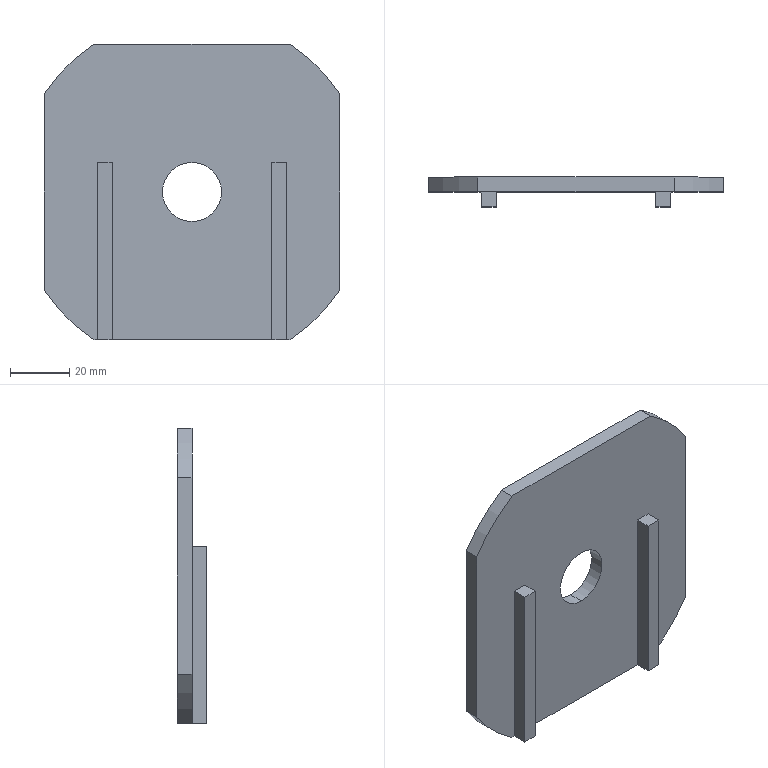Part | STEP file | Guide wheel mechanism revised.sldasm-Part-348 | 1 solid | 20 faces | box 100 x 10 x 100 mm | volume 48975 mm3 | plane 14 | cylinder 6 | commonest cylinder face diameters 120 x4 20 x2
STEP:
#1=CARTESIAN_POINT('',(0.,5.,-10.));
#2=VERTEX_POINT('',#1);
#3=CARTESIAN_POINT('',(0.,5.,10.));
#4=VERTEX_POINT('',#3);
#5=CARTESIAN_POINT('',(0.,5.,0.));
#6=DIRECTION('',(0.,1.,0.));
#7=DIRECTION('',(0.,0.,1.));
#8=AXIS2_PLACEMENT_3D('',#5,#6,#7);
#9=CIRCLE('',#8,10.);
#10=EDGE_CURVE('',#2,#4,#9,.T.);
#11=ORIENTED_EDGE('',*,*,#10,.T.);
#12=CARTESIAN_POINT('',(0.,0.,10.));
#13=VERTEX_POINT('',#12);
#14=CARTESIAN_POINT('',(0.,5.,10.));
#15=DIRECTION('',(0.,-1.,0.));
#16=VECTOR('',#15,1000.);
#17=LINE('',#14,#16);
#18=EDGE_CURVE('',#4,#13,#17,.T.);
#19=ORIENTED_EDGE('',*,*,#18,.T.);
#20=CARTESIAN_POINT('',(0.,0.,-10.));
#21=VERTEX_POINT('',#20);
#22=CARTESIAN_POINT('',(0.,0.,0.));
#23=DIRECTION('',(0.,1.,0.));
#24=DIRECTION('',(0.,0.,1.));
#25=AXIS2_PLACEMENT_3D('',#22,#23,#24);
#26=CIRCLE('',#25,10.);
#27=EDGE_CURVE('',#21,#13,#26,.T.);
#28=ORIENTED_EDGE('',*,*,#27,.F.);
#29=CARTESIAN_POINT('',(0.,5.,-10.));
#30=DIRECTION('',(0.,-1.,0.));
#31=VECTOR('',#30,1000.);
#32=LINE('',#29,#31);
#33=EDGE_CURVE('',#2,#21,#32,.T.);
#34=ORIENTED_EDGE('',*,*,#33,.F.);
#35=EDGE_LOOP('',(#11,#19,#28,#34));
#36=FACE_OUTER_BOUND('',#35,.T.);
#37=CARTESIAN_POINT('',(0.,5.,0.));
#38=DIRECTION('',(0.,-1.,0.));
#39=DIRECTION('',(0.,0.,-1.));
#40=AXIS2_PLACEMENT_3D('',#37,#38,#39);
#41=CYLINDRICAL_SURFACE('',#40,10.);
#42=ADVANCED_FACE('',(#36),#41,.F.);
#43=ORIENTED_EDGE('',*,*,#10,.F.);
#44=CARTESIAN_POINT('',(0.,5.,0.));
#45=DIRECTION('',(0.,1.,0.));
#46=DIRECTION('',(0.,0.,1.));
#47=AXIS2_PLACEMENT_3D('',#44,#45,#46);
#48=CIRCLE('',#47,10.);
#49=EDGE_CURVE('',#4,#2,#48,.T.);
#50=ORIENTED_EDGE('',*,*,#49,.F.);
#51=EDGE_LOOP('',(#43,#50));
#52=FACE_BOUND('',#51,.T.);
#53=CARTESIAN_POINT('',(-33.166,5.,50.));
#54=VERTEX_POINT('',#53);
#55=CARTESIAN_POINT('',(33.166,5.,50.));
#56=VERTEX_POINT('',#55);
#57=CARTESIAN_POINT('',(50.,5.,50.));
#58=DIRECTION('',(1.,0.,0.));
#59=VECTOR('',#58,1000.);
#60=LINE('',#57,#59);
#61=EDGE_CURVE('',#54,#56,#60,.T.);
#62=ORIENTED_EDGE('',*,*,#61,.T.);
#63=CARTESIAN_POINT('',(50.,5.,33.166));
#64=VERTEX_POINT('',#63);
#65=CARTESIAN_POINT('',(0.,5.,0.));
#66=DIRECTION('',(0.,1.,0.));
#67=DIRECTION('',(0.,0.,1.));
#68=AXIS2_PLACEMENT_3D('',#65,#66,#67);
#69=CIRCLE('',#68,60.);
#70=EDGE_CURVE('',#56,#64,#69,.T.);
#71=ORIENTED_EDGE('',*,*,#70,.T.);
#72=CARTESIAN_POINT('',(50.,5.,-33.166));
#73=VERTEX_POINT('',#72);
#74=CARTESIAN_POINT('',(50.,5.,50.));
#75=DIRECTION('',(0.,0.,-1.));
#76=VECTOR('',#75,1000.);
#77=LINE('',#74,#76);
#78=EDGE_CURVE('',#64,#73,#77,.T.);
#79=ORIENTED_EDGE('',*,*,#78,.T.);
#80=CARTESIAN_POINT('',(33.166,5.,-50.));
#81=VERTEX_POINT('',#80);
#82=CARTESIAN_POINT('',(0.,5.,0.));
#83=DIRECTION('',(0.,1.,0.));
#84=DIRECTION('',(0.,0.,1.));
#85=AXIS2_PLACEMENT_3D('',#82,#83,#84);
#86=CIRCLE('',#85,60.);
#87=EDGE_CURVE('',#73,#81,#86,.T.);
#88=ORIENTED_EDGE('',*,*,#87,.T.);
#89=CARTESIAN_POINT('',(-33.166,5.,-50.));
#90=VERTEX_POINT('',#89);
#91=CARTESIAN_POINT('',(50.,5.,-50.));
#92=DIRECTION('',(-1.,0.,0.));
#93=VECTOR('',#92,1000.);
#94=LINE('',#91,#93);
#95=EDGE_CURVE('',#81,#90,#94,.T.);
#96=ORIENTED_EDGE('',*,*,#95,.T.);
#97=CARTESIAN_POINT('',(-50.,5.,-33.166));
#98=VERTEX_POINT('',#97);
#99=CARTESIAN_POINT('',(0.,5.,0.));
#100=DIRECTION('',(0.,1.,0.));
#101=DIRECTION('',(0.,0.,1.));
#102=AXIS2_PLACEMENT_3D('',#99,#100,#101);
#103=CIRCLE('',#102,60.);
#104=EDGE_CURVE('',#90,#98,#103,.T.);
#105=ORIENTED_EDGE('',*,*,#104,.T.);
#106=CARTESIAN_POINT('',(-50.,5.,33.166));
#107=VERTEX_POINT('',#106);
#108=CARTESIAN_POINT('',(-50.,5.,50.));
#109=DIRECTION('',(0.,0.,1.));
#110=VECTOR('',#109,1000.);
#111=LINE('',#108,#110);
#112=EDGE_CURVE('',#98,#107,#111,.T.);
#113=ORIENTED_EDGE('',*,*,#112,.T.);
#114=CARTESIAN_POINT('',(0.,5.,0.));
#115=DIRECTION('',(0.,1.,0.));
#116=DIRECTION('',(0.,0.,1.));
#117=AXIS2_PLACEMENT_3D('',#114,#115,#116);
#118=CIRCLE('',#117,60.);
#119=EDGE_CURVE('',#107,#54,#118,.T.);
#120=ORIENTED_EDGE('',*,*,#119,.T.);
#121=EDGE_LOOP('',(#62,#71,#79,#88,#96,#105,#113,#120));
#122=FACE_OUTER_BOUND('',#121,.T.);
#123=CARTESIAN_POINT('',(0.,5.,0.));
#124=DIRECTION('',(0.,1.,0.));
#125=DIRECTION('',(0.,0.,1.));
#126=AXIS2_PLACEMENT_3D('',#123,#124,#125);
#127=PLANE('',#126);
#128=ADVANCED_FACE('',(#52,#122),#127,.T.);
#129=CARTESIAN_POINT('',(27.,0.,-50.));
#130=VERTEX_POINT('',#129);
#131=CARTESIAN_POINT('',(-27.,0.,-50.));
#132=VERTEX_POINT('',#131);
#133=CARTESIAN_POINT('',(50.,0.,-50.));
#134=DIRECTION('',(-1.,0.,0.));
#135=VECTOR('',#134,1000.);
#136=LINE('',#133,#135);
#137=EDGE_CURVE('',#130,#132,#136,.T.);
#138=ORIENTED_EDGE('',*,*,#137,.F.);
#139=CARTESIAN_POINT('',(27.,0.,10.));
#140=VERTEX_POINT('',#139);
#141=CARTESIAN_POINT('',(27.,0.,-50.));
#142=DIRECTION('',(0.,0.,1.));
#143=VECTOR('',#142,1000.);
#144=LINE('',#141,#143);
#145=EDGE_CURVE('',#130,#140,#144,.T.);
#146=ORIENTED_EDGE('',*,*,#145,.T.);
#147=CARTESIAN_POINT('',(32.,0.,10.));
#148=VERTEX_POINT('',#147);
#149=CARTESIAN_POINT('',(27.,0.,10.));
#150=DIRECTION('',(1.,0.,0.));
#151=VECTOR('',#150,1000.);
#152=LINE('',#149,#151);
#153=EDGE_CURVE('',#140,#148,#152,.T.);
#154=ORIENTED_EDGE('',*,*,#153,.T.);
#155=CARTESIAN_POINT('',(32.,0.,-50.));
#156=VERTEX_POINT('',#155);
#157=CARTESIAN_POINT('',(32.,0.,-50.));
#158=DIRECTION('',(0.,0.,-1.));
#159=VECTOR('',#158,1000.);
#160=LINE('',#157,#159);
#161=EDGE_CURVE('',#148,#156,#160,.T.);
#162=ORIENTED_EDGE('',*,*,#161,.T.);
#163=CARTESIAN_POINT('',(33.166,0.,-50.));
#164=VERTEX_POINT('',#163);
#165=CARTESIAN_POINT('',(50.,0.,-50.));
#166=DIRECTION('',(-1.,0.,0.));
#167=VECTOR('',#166,1000.);
#168=LINE('',#165,#167);
#169=EDGE_CURVE('',#164,#156,#168,.T.);
#170=ORIENTED_EDGE('',*,*,#169,.F.);
#171=CARTESIAN_POINT('',(50.,0.,-33.166));
#172=VERTEX_POINT('',#171);
#173=CARTESIAN_POINT('',(0.,0.,0.));
#174=DIRECTION('',(0.,1.,0.));
#175=DIRECTION('',(0.,0.,1.));
#176=AXIS2_PLACEMENT_3D('',#173,#174,#175);
#177=CIRCLE('',#176,60.);
#178=EDGE_CURVE('',#172,#164,#177,.T.);
#179=ORIENTED_EDGE('',*,*,#178,.F.);
#180=CARTESIAN_POINT('',(50.,0.,33.166));
#181=VERTEX_POINT('',#180);
#182=CARTESIAN_POINT('',(50.,0.,50.));
#183=DIRECTION('',(0.,0.,-1.));
#184=VECTOR('',#183,1000.);
#185=LINE('',#182,#184);
#186=EDGE_CURVE('',#181,#172,#185,.T.);
#187=ORIENTED_EDGE('',*,*,#186,.F.);
#188=CARTESIAN_POINT('',(33.166,0.,50.));
#189=VERTEX_POINT('',#188);
#190=CARTESIAN_POINT('',(0.,0.,0.));
#191=DIRECTION('',(0.,1.,0.));
#192=DIRECTION('',(0.,0.,1.));
#193=AXIS2_PLACEMENT_3D('',#190,#191,#192);
#194=CIRCLE('',#193,60.);
#195=EDGE_CURVE('',#189,#181,#194,.T.);
#196=ORIENTED_EDGE('',*,*,#195,.F.);
#197=CARTESIAN_POINT('',(-33.166,0.,50.));
#198=VERTEX_POINT('',#197);
#199=CARTESIAN_POINT('',(50.,0.,50.));
#200=DIRECTION('',(1.,0.,0.));
#201=VECTOR('',#200,1000.);
#202=LINE('',#199,#201);
#203=EDGE_CURVE('',#198,#189,#202,.T.);
#204=ORIENTED_EDGE('',*,*,#203,.F.);
#205=CARTESIAN_POINT('',(-50.,0.,33.166));
#206=VERTEX_POINT('',#205);
#207=CARTESIAN_POINT('',(0.,0.,0.));
#208=DIRECTION('',(0.,1.,0.));
#209=DIRECTION('',(0.,0.,1.));
#210=AXIS2_PLACEMENT_3D('',#207,#208,#209);
#211=CIRCLE('',#210,60.);
#212=EDGE_CURVE('',#206,#198,#211,.T.);
#213=ORIENTED_EDGE('',*,*,#212,.F.);
#214=CARTESIAN_POINT('',(-50.,0.,-33.166));
#215=VERTEX_POINT('',#214);
#216=CARTESIAN_POINT('',(-50.,0.,50.));
#217=DIRECTION('',(0.,0.,1.));
#218=VECTOR('',#217,1000.);
#219=LINE('',#216,#218);
#220=EDGE_CURVE('',#215,#206,#219,.T.);
#221=ORIENTED_EDGE('',*,*,#220,.F.);
#222=CARTESIAN_POINT('',(-33.166,0.,-50.));
#223=VERTEX_POINT('',#222);
#224=CARTESIAN_POINT('',(0.,0.,0.));
#225=DIRECTION('',(0.,1.,0.));
#226=DIRECTION('',(0.,0.,1.));
#227=AXIS2_PLACEMENT_3D('',#224,#225,#226);
#228=CIRCLE('',#227,60.);
#229=EDGE_CURVE('',#223,#215,#228,.T.);
#230=ORIENTED_EDGE('',*,*,#229,.F.);
#231=CARTESIAN_POINT('',(-32.,0.,-50.));
#232=VERTEX_POINT('',#231);
#233=CARTESIAN_POINT('',(50.,0.,-50.));
#234=DIRECTION('',(-1.,0.,0.));
#235=VECTOR('',#234,1000.);
#236=LINE('',#233,#235);
#237=EDGE_CURVE('',#232,#223,#236,.T.);
#238=ORIENTED_EDGE('',*,*,#237,.F.);
#239=CARTESIAN_POINT('',(-32.,0.,10.));
#240=VERTEX_POINT('',#239);
#241=CARTESIAN_POINT('',(-32.,0.,-50.));
#242=DIRECTION('',(0.,0.,1.));
#243=VECTOR('',#242,1000.);
#244=LINE('',#241,#243);
#245=EDGE_CURVE('',#232,#240,#244,.T.);
#246=ORIENTED_EDGE('',*,*,#245,.T.);
#247=CARTESIAN_POINT('',(-27.,0.,10.));
#248=VERTEX_POINT('',#247);
#249=CARTESIAN_POINT('',(-32.,0.,10.));
#250=DIRECTION('',(1.,0.,0.));
#251=VECTOR('',#250,1000.);
#252=LINE('',#249,#251);
#253=EDGE_CURVE('',#240,#248,#252,.T.);
#254=ORIENTED_EDGE('',*,*,#253,.T.);
#255=CARTESIAN_POINT('',(-27.,0.,-50.));
#256=DIRECTION('',(0.,0.,-1.));
#257=VECTOR('',#256,1000.);
#258=LINE('',#255,#257);
#259=EDGE_CURVE('',#248,#132,#258,.T.);
#260=ORIENTED_EDGE('',*,*,#259,.T.);
#261=EDGE_LOOP('',(#138,#146,#154,#162,#170,#179,#187,#196,#204,#213,#221,#230,#238,#246,#254,#260));
#262=FACE_OUTER_BOUND('',#261,.T.);
#263=ORIENTED_EDGE('',*,*,#27,.T.);
#264=CARTESIAN_POINT('',(0.,0.,0.));
#265=DIRECTION('',(0.,1.,0.));
#266=DIRECTION('',(0.,0.,1.));
#267=AXIS2_PLACEMENT_3D('',#264,#265,#266);
#268=CIRCLE('',#267,10.);
#269=EDGE_CURVE('',#13,#21,#268,.T.);
#270=ORIENTED_EDGE('',*,*,#269,.T.);
#271=EDGE_LOOP('',(#263,#270));
#272=FACE_BOUND('',#271,.T.);
#273=CARTESIAN_POINT('',(0.,0.,0.));
#274=DIRECTION('',(0.,1.,0.));
#275=DIRECTION('',(0.,0.,1.));
#276=AXIS2_PLACEMENT_3D('',#273,#274,#275);
#277=PLANE('',#276);
#278=ADVANCED_FACE('',(#262,#272),#277,.F.);
#279=CARTESIAN_POINT('',(-50.,-5.,-33.166));
#280=DIRECTION('',(0.,1.,0.));
#281=VECTOR('',#280,1000.);
#282=LINE('',#279,#281);
#283=EDGE_CURVE('',#215,#98,#282,.T.);
#284=ORIENTED_EDGE('',*,*,#283,.F.);
#285=ORIENTED_EDGE('',*,*,#220,.T.);
#286=CARTESIAN_POINT('',(-50.,-5.,33.166));
#287=DIRECTION('',(0.,-1.,0.));
#288=VECTOR('',#287,1000.);
#289=LINE('',#286,#288);
#290=EDGE_CURVE('',#107,#206,#289,.T.);
#291=ORIENTED_EDGE('',*,*,#290,.F.);
#292=ORIENTED_EDGE('',*,*,#112,.F.);
#293=EDGE_LOOP('',(#284,#285,#291,#292));
#294=FACE_OUTER_BOUND('',#293,.T.);
#295=CARTESIAN_POINT('',(-50.,5.,50.));
#296=DIRECTION('',(1.,0.,0.));
#297=DIRECTION('',(0.,0.,-1.));
#298=AXIS2_PLACEMENT_3D('',#295,#296,#297);
#299=PLANE('',#298);
#300=ADVANCED_FACE('',(#294),#299,.F.);
#301=CARTESIAN_POINT('',(-33.166,-5.,50.));
#302=DIRECTION('',(0.,1.,0.));
#303=VECTOR('',#302,1000.);
#304=LINE('',#301,#303);
#305=EDGE_CURVE('',#198,#54,#304,.T.);
#306=ORIENTED_EDGE('',*,*,#305,.F.);
#307=ORIENTED_EDGE('',*,*,#203,.T.);
#308=CARTESIAN_POINT('',(33.166,-5.,50.));
#309=DIRECTION('',(0.,-1.,0.));
#310=VECTOR('',#309,1000.);
#311=LINE('',#308,#310);
#312=EDGE_CURVE('',#56,#189,#311,.T.);
#313=ORIENTED_EDGE('',*,*,#312,.F.);
#314=ORIENTED_EDGE('',*,*,#61,.F.);
#315=EDGE_LOOP('',(#306,#307,#313,#314));
#316=FACE_OUTER_BOUND('',#315,.T.);
#317=CARTESIAN_POINT('',(50.,5.,50.));
#318=DIRECTION('',(0.,0.,-1.));
#319=DIRECTION('',(-1.,0.,0.));
#320=AXIS2_PLACEMENT_3D('',#317,#318,#319);
#321=PLANE('',#320);
#322=ADVANCED_FACE('',(#316),#321,.F.);
#323=CARTESIAN_POINT('',(50.,-5.,33.166));
#324=DIRECTION('',(0.,1.,0.));
#325=VECTOR('',#324,1000.);
#326=LINE('',#323,#325);
#327=EDGE_CURVE('',#181,#64,#326,.T.);
#328=ORIENTED_EDGE('',*,*,#327,.F.);
#329=ORIENTED_EDGE('',*,*,#186,.T.);
#330=CARTESIAN_POINT('',(50.,-5.,-33.166));
#331=DIRECTION('',(0.,-1.,0.));
#332=VECTOR('',#331,1000.);
#333=LINE('',#330,#332);
#334=EDGE_CURVE('',#73,#172,#333,.T.);
#335=ORIENTED_EDGE('',*,*,#334,.F.);
#336=ORIENTED_EDGE('',*,*,#78,.F.);
#337=EDGE_LOOP('',(#328,#329,#335,#336));
#338=FACE_OUTER_BOUND('',#337,.T.);
#339=CARTESIAN_POINT('',(50.,5.,50.));
#340=DIRECTION('',(-1.,0.,0.));
#341=DIRECTION('',(0.,0.,1.));
#342=AXIS2_PLACEMENT_3D('',#339,#340,#341);
#343=PLANE('',#342);
#344=ADVANCED_FACE('',(#338),#343,.F.);
#345=CARTESIAN_POINT('',(33.166,-5.,-50.));
#346=DIRECTION('',(0.,1.,0.));
#347=VECTOR('',#346,1000.);
#348=LINE('',#345,#347);
#349=EDGE_CURVE('',#164,#81,#348,.T.);
#350=ORIENTED_EDGE('',*,*,#349,.F.);
#351=ORIENTED_EDGE('',*,*,#169,.T.);
#352=CARTESIAN_POINT('',(32.,-5.,-50.));
#353=VERTEX_POINT('',#352);
#354=CARTESIAN_POINT('',(32.,-5.,-50.));
#355=DIRECTION('',(0.,1.,0.));
#356=VECTOR('',#355,1000.);
#357=LINE('',#354,#356);
#358=EDGE_CURVE('',#353,#156,#357,.T.);
#359=ORIENTED_EDGE('',*,*,#358,.F.);
#360=CARTESIAN_POINT('',(27.,-5.,-50.));
#361=VERTEX_POINT('',#360);
#362=CARTESIAN_POINT('',(27.,-5.,-50.));
#363=DIRECTION('',(-1.,0.,0.));
#364=VECTOR('',#363,1000.);
#365=LINE('',#362,#364);
#366=EDGE_CURVE('',#353,#361,#365,.T.);
#367=ORIENTED_EDGE('',*,*,#366,.T.);
#368=CARTESIAN_POINT('',(27.,-5.,-50.));
#369=DIRECTION('',(0.,1.,0.));
#370=VECTOR('',#369,1000.);
#371=LINE('',#368,#370);
#372=EDGE_CURVE('',#361,#130,#371,.T.);
#373=ORIENTED_EDGE('',*,*,#372,.T.);
#374=ORIENTED_EDGE('',*,*,#137,.T.);
#375=CARTESIAN_POINT('',(-27.,-5.,-50.));
#376=VERTEX_POINT('',#375);
#377=CARTESIAN_POINT('',(-27.,-5.,-50.));
#378=DIRECTION('',(0.,1.,0.));
#379=VECTOR('',#378,1000.);
#380=LINE('',#377,#379);
#381=EDGE_CURVE('',#376,#132,#380,.T.);
#382=ORIENTED_EDGE('',*,*,#381,.F.);
#383=CARTESIAN_POINT('',(-32.,-5.,-50.));
#384=VERTEX_POINT('',#383);
#385=CARTESIAN_POINT('',(-32.,-5.,-50.));
#386=DIRECTION('',(-1.,0.,0.));
#387=VECTOR('',#386,1000.);
#388=LINE('',#385,#387);
#389=EDGE_CURVE('',#376,#384,#388,.T.);
#390=ORIENTED_EDGE('',*,*,#389,.T.);
#391=CARTESIAN_POINT('',(-32.,-5.,-50.));
#392=DIRECTION('',(0.,1.,0.));
#393=VECTOR('',#392,1000.);
#394=LINE('',#391,#393);
#395=EDGE_CURVE('',#384,#232,#394,.T.);
#396=ORIENTED_EDGE('',*,*,#395,.T.);
#397=ORIENTED_EDGE('',*,*,#237,.T.);
#398=CARTESIAN_POINT('',(-33.166,-5.,-50.));
#399=DIRECTION('',(0.,-1.,0.));
#400=VECTOR('',#399,1000.);
#401=LINE('',#398,#400);
#402=EDGE_CURVE('',#90,#223,#401,.T.);
#403=ORIENTED_EDGE('',*,*,#402,.F.);
#404=ORIENTED_EDGE('',*,*,#95,.F.);
#405=EDGE_LOOP('',(#350,#351,#359,#367,#373,#374,#382,#390,#396,#397,#403,#404));
#406=FACE_OUTER_BOUND('',#405,.T.);
#407=CARTESIAN_POINT('',(50.,5.,-50.));
#408=DIRECTION('',(0.,0.,1.));
#409=DIRECTION('',(1.,0.,0.));
#410=AXIS2_PLACEMENT_3D('',#407,#408,#409);
#411=PLANE('',#410);
#412=ADVANCED_FACE('',(#406),#411,.F.);
#413=ORIENTED_EDGE('',*,*,#18,.F.);
#414=ORIENTED_EDGE('',*,*,#49,.T.);
#415=ORIENTED_EDGE('',*,*,#33,.T.);
#416=ORIENTED_EDGE('',*,*,#269,.F.);
#417=EDGE_LOOP('',(#413,#414,#415,#416));
#418=FACE_OUTER_BOUND('',#417,.T.);
#419=CARTESIAN_POINT('',(0.,5.,0.));
#420=DIRECTION('',(0.,-1.,0.));
#421=DIRECTION('',(0.,0.,-1.));
#422=AXIS2_PLACEMENT_3D('',#419,#420,#421);
#423=CYLINDRICAL_SURFACE('',#422,10.);
#424=ADVANCED_FACE('',(#418),#423,.F.);
#425=ORIENTED_EDGE('',*,*,#283,.T.);
#426=ORIENTED_EDGE('',*,*,#104,.F.);
#427=ORIENTED_EDGE('',*,*,#402,.T.);
#428=ORIENTED_EDGE('',*,*,#229,.T.);
#429=EDGE_LOOP('',(#425,#426,#427,#428));
#430=FACE_OUTER_BOUND('',#429,.T.);
#431=CARTESIAN_POINT('',(0.,-5.,0.));
#432=DIRECTION('',(0.,1.,0.));
#433=DIRECTION('',(0.,0.,1.));
#434=AXIS2_PLACEMENT_3D('',#431,#432,#433);
#435=CYLINDRICAL_SURFACE('',#434,60.);
#436=ADVANCED_FACE('',(#430),#435,.T.);
#437=ORIENTED_EDGE('',*,*,#334,.T.);
#438=ORIENTED_EDGE('',*,*,#178,.T.);
#439=ORIENTED_EDGE('',*,*,#349,.T.);
#440=ORIENTED_EDGE('',*,*,#87,.F.);
#441=EDGE_LOOP('',(#437,#438,#439,#440));
#442=FACE_OUTER_BOUND('',#441,.T.);
#443=CARTESIAN_POINT('',(0.,-5.,0.));
#444=DIRECTION('',(0.,1.,0.));
#445=DIRECTION('',(0.,0.,1.));
#446=AXIS2_PLACEMENT_3D('',#443,#444,#445);
#447=CYLINDRICAL_SURFACE('',#446,60.);
#448=ADVANCED_FACE('',(#442),#447,.T.);
#449=ORIENTED_EDGE('',*,*,#312,.T.);
#450=ORIENTED_EDGE('',*,*,#195,.T.);
#451=ORIENTED_EDGE('',*,*,#327,.T.);
#452=ORIENTED_EDGE('',*,*,#70,.F.);
#453=EDGE_LOOP('',(#449,#450,#451,#452));
#454=FACE_OUTER_BOUND('',#453,.T.);
#455=CARTESIAN_POINT('',(0.,-5.,0.));
#456=DIRECTION('',(0.,1.,0.));
#457=DIRECTION('',(0.,0.,1.));
#458=AXIS2_PLACEMENT_3D('',#455,#456,#457);
#459=CYLINDRICAL_SURFACE('',#458,60.);
#460=ADVANCED_FACE('',(#454),#459,.T.);
#461=ORIENTED_EDGE('',*,*,#290,.T.);
#462=ORIENTED_EDGE('',*,*,#212,.T.);
#463=ORIENTED_EDGE('',*,*,#305,.T.);
#464=ORIENTED_EDGE('',*,*,#119,.F.);
#465=EDGE_LOOP('',(#461,#462,#463,#464));
#466=FACE_OUTER_BOUND('',#465,.T.);
#467=CARTESIAN_POINT('',(0.,-5.,0.));
#468=DIRECTION('',(0.,1.,0.));
#469=DIRECTION('',(0.,0.,1.));
#470=AXIS2_PLACEMENT_3D('',#467,#468,#469);
#471=CYLINDRICAL_SURFACE('',#470,60.);
#472=ADVANCED_FACE('',(#466),#471,.T.);
#473=ORIENTED_EDGE('',*,*,#245,.F.);
#474=ORIENTED_EDGE('',*,*,#395,.F.);
#475=CARTESIAN_POINT('',(-32.,-5.,10.));
#476=VERTEX_POINT('',#475);
#477=CARTESIAN_POINT('',(-32.,-5.,-50.));
#478=DIRECTION('',(0.,0.,1.));
#479=VECTOR('',#478,1000.);
#480=LINE('',#477,#479);
#481=EDGE_CURVE('',#384,#476,#480,.T.);
#482=ORIENTED_EDGE('',*,*,#481,.T.);
#483=CARTESIAN_POINT('',(-32.,-5.,10.));
#484=DIRECTION('',(0.,1.,0.));
#485=VECTOR('',#484,1000.);
#486=LINE('',#483,#485);
#487=EDGE_CURVE('',#476,#240,#486,.T.);
#488=ORIENTED_EDGE('',*,*,#487,.T.);
#489=EDGE_LOOP('',(#473,#474,#482,#488));
#490=FACE_OUTER_BOUND('',#489,.T.);
#491=CARTESIAN_POINT('',(-32.,-5.,-50.));
#492=DIRECTION('',(-1.,0.,0.));
#493=DIRECTION('',(0.,0.,1.));
#494=AXIS2_PLACEMENT_3D('',#491,#492,#493);
#495=PLANE('',#494);
#496=ADVANCED_FACE('',(#490),#495,.T.);
#497=ORIENTED_EDGE('',*,*,#259,.F.);
#498=CARTESIAN_POINT('',(-27.,-5.,10.));
#499=VERTEX_POINT('',#498);
#500=CARTESIAN_POINT('',(-27.,-5.,10.));
#501=DIRECTION('',(0.,1.,0.));
#502=VECTOR('',#501,1000.);
#503=LINE('',#500,#502);
#504=EDGE_CURVE('',#499,#248,#503,.T.);
#505=ORIENTED_EDGE('',*,*,#504,.F.);
#506=CARTESIAN_POINT('',(-27.,-5.,-50.));
#507=DIRECTION('',(0.,0.,-1.));
#508=VECTOR('',#507,1000.);
#509=LINE('',#506,#508);
#510=EDGE_CURVE('',#499,#376,#509,.T.);
#511=ORIENTED_EDGE('',*,*,#510,.T.);
#512=ORIENTED_EDGE('',*,*,#381,.T.);
#513=EDGE_LOOP('',(#497,#505,#511,#512));
#514=FACE_OUTER_BOUND('',#513,.T.);
#515=CARTESIAN_POINT('',(-27.,-5.,-50.));
#516=DIRECTION('',(1.,0.,0.));
#517=DIRECTION('',(0.,0.,-1.));
#518=AXIS2_PLACEMENT_3D('',#515,#516,#517);
#519=PLANE('',#518);
#520=ADVANCED_FACE('',(#514),#519,.T.);
#521=ORIENTED_EDGE('',*,*,#253,.F.);
#522=ORIENTED_EDGE('',*,*,#487,.F.);
#523=CARTESIAN_POINT('',(-32.,-5.,10.));
#524=DIRECTION('',(1.,0.,0.));
#525=VECTOR('',#524,1000.);
#526=LINE('',#523,#525);
#527=EDGE_CURVE('',#476,#499,#526,.T.);
#528=ORIENTED_EDGE('',*,*,#527,.T.);
#529=ORIENTED_EDGE('',*,*,#504,.T.);
#530=EDGE_LOOP('',(#521,#522,#528,#529));
#531=FACE_OUTER_BOUND('',#530,.T.);
#532=CARTESIAN_POINT('',(-32.,-5.,10.));
#533=DIRECTION('',(0.,0.,1.));
#534=DIRECTION('',(1.,0.,0.));
#535=AXIS2_PLACEMENT_3D('',#532,#533,#534);
#536=PLANE('',#535);
#537=ADVANCED_FACE('',(#531),#536,.T.);
#538=ORIENTED_EDGE('',*,*,#481,.F.);
#539=ORIENTED_EDGE('',*,*,#389,.F.);
#540=ORIENTED_EDGE('',*,*,#510,.F.);
#541=ORIENTED_EDGE('',*,*,#527,.F.);
#542=EDGE_LOOP('',(#538,#539,#540,#541));
#543=FACE_OUTER_BOUND('',#542,.T.);
#544=CARTESIAN_POINT('',(0.,-5.,0.));
#545=DIRECTION('',(0.,1.,0.));
#546=DIRECTION('',(0.,0.,1.));
#547=AXIS2_PLACEMENT_3D('',#544,#545,#546);
#548=PLANE('',#547);
#549=ADVANCED_FACE('',(#543),#548,.F.);
#550=ORIENTED_EDGE('',*,*,#145,.F.);
#551=ORIENTED_EDGE('',*,*,#372,.F.);
#552=CARTESIAN_POINT('',(27.,-5.,10.));
#553=VERTEX_POINT('',#552);
#554=CARTESIAN_POINT('',(27.,-5.,-50.));
#555=DIRECTION('',(0.,0.,1.));
#556=VECTOR('',#555,1000.);
#557=LINE('',#554,#556);
#558=EDGE_CURVE('',#361,#553,#557,.T.);
#559=ORIENTED_EDGE('',*,*,#558,.T.);
#560=CARTESIAN_POINT('',(27.,-5.,10.));
#561=DIRECTION('',(0.,1.,0.));
#562=VECTOR('',#561,1000.);
#563=LINE('',#560,#562);
#564=EDGE_CURVE('',#553,#140,#563,.T.);
#565=ORIENTED_EDGE('',*,*,#564,.T.);
#566=EDGE_LOOP('',(#550,#551,#559,#565));
#567=FACE_OUTER_BOUND('',#566,.T.);
#568=CARTESIAN_POINT('',(27.,-5.,-50.));
#569=DIRECTION('',(-1.,0.,0.));
#570=DIRECTION('',(0.,0.,1.));
#571=AXIS2_PLACEMENT_3D('',#568,#569,#570);
#572=PLANE('',#571);
#573=ADVANCED_FACE('',(#567),#572,.T.);
#574=ORIENTED_EDGE('',*,*,#161,.F.);
#575=CARTESIAN_POINT('',(32.,-5.,10.));
#576=VERTEX_POINT('',#575);
#577=CARTESIAN_POINT('',(32.,-5.,10.));
#578=DIRECTION('',(0.,1.,0.));
#579=VECTOR('',#578,1000.);
#580=LINE('',#577,#579);
#581=EDGE_CURVE('',#576,#148,#580,.T.);
#582=ORIENTED_EDGE('',*,*,#581,.F.);
#583=CARTESIAN_POINT('',(32.,-5.,-50.));
#584=DIRECTION('',(0.,0.,-1.));
#585=VECTOR('',#584,1000.);
#586=LINE('',#583,#585);
#587=EDGE_CURVE('',#576,#353,#586,.T.);
#588=ORIENTED_EDGE('',*,*,#587,.T.);
#589=ORIENTED_EDGE('',*,*,#358,.T.);
#590=EDGE_LOOP('',(#574,#582,#588,#589));
#591=FACE_OUTER_BOUND('',#590,.T.);
#592=CARTESIAN_POINT('',(32.,-5.,-50.));
#593=DIRECTION('',(1.,0.,0.));
#594=DIRECTION('',(0.,0.,-1.));
#595=AXIS2_PLACEMENT_3D('',#592,#593,#594);
#596=PLANE('',#595);
#597=ADVANCED_FACE('',(#591),#596,.T.);
#598=ORIENTED_EDGE('',*,*,#153,.F.);
#599=ORIENTED_EDGE('',*,*,#564,.F.);
#600=CARTESIAN_POINT('',(27.,-5.,10.));
#601=DIRECTION('',(1.,0.,0.));
#602=VECTOR('',#601,1000.);
#603=LINE('',#600,#602);
#604=EDGE_CURVE('',#553,#576,#603,.T.);
#605=ORIENTED_EDGE('',*,*,#604,.T.);
#606=ORIENTED_EDGE('',*,*,#581,.T.);
#607=EDGE_LOOP('',(#598,#599,#605,#606));
#608=FACE_OUTER_BOUND('',#607,.T.);
#609=CARTESIAN_POINT('',(27.,-5.,10.));
#610=DIRECTION('',(0.,0.,1.));
#611=DIRECTION('',(1.,0.,0.));
#612=AXIS2_PLACEMENT_3D('',#609,#610,#611);
#613=PLANE('',#612);
#614=ADVANCED_FACE('',(#608),#613,.T.);
#615=ORIENTED_EDGE('',*,*,#558,.F.);
#616=ORIENTED_EDGE('',*,*,#366,.F.);
#617=ORIENTED_EDGE('',*,*,#587,.F.);
#618=ORIENTED_EDGE('',*,*,#604,.F.);
#619=EDGE_LOOP('',(#615,#616,#617,#618));
#620=FACE_OUTER_BOUND('',#619,.T.);
#621=CARTESIAN_POINT('',(0.,-5.,0.));
#622=DIRECTION('',(0.,1.,0.));
#623=DIRECTION('',(0.,0.,1.));
#624=AXIS2_PLACEMENT_3D('',#621,#622,#623);
#625=PLANE('',#624);
#626=ADVANCED_FACE('',(#620),#625,.F.);
#627=CLOSED_SHELL('',(#42,#128,#278,#300,#322,#344,#412,#424,#436,#448,#460,#472,#496,#520,#537,#549,#573,#597,#614,#626));
#628=MANIFOLD_SOLID_BREP('',#627);
#629=CARTESIAN_POINT('',(0.,0.,0.));
#630=DIRECTION('',(0.,0.,1.));
#631=DIRECTION('',(1.,0.,0.));
#632=AXIS2_PLACEMENT_3D('',#629,#630,#631);
#633=(LENGTH_UNIT()NAMED_UNIT(*)SI_UNIT(.MILLI.,.METRE.));
#634=UNCERTAINTY_MEASURE_WITH_UNIT(LENGTH_MEASURE(0.00001),#633,'','');
#635=(NAMED_UNIT(*)PLANE_ANGLE_UNIT()SI_UNIT($,.RADIAN.));
#636=(NAMED_UNIT(*)SI_UNIT($,.STERADIAN.)SOLID_ANGLE_UNIT());
#637=(GEOMETRIC_REPRESENTATION_CONTEXT(3)GLOBAL_UNCERTAINTY_ASSIGNED_CONTEXT((#634))GLOBAL_UNIT_ASSIGNED_CONTEXT((#633,#635,#636))REPRESENTATION_CONTEXT('',''));
#638=ADVANCED_BREP_SHAPE_REPRESENTATION('',(#628,#632),#637);